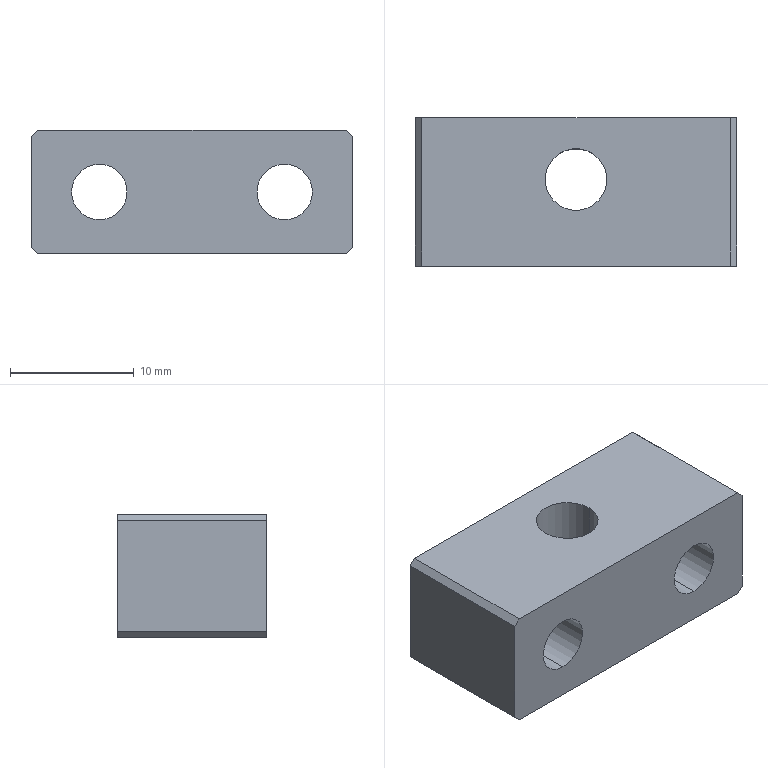Part | SolidWorks | features HoleWzd 2, Chamfer 1, Extrusion 1 | 1 solid | 22 faces | box 26 x 12 x 10 mm | volume 2220 mm3 | plane 12 | cylinder 10 | commonest cylinder face diameters 4.5 x4 8 x4 5 x2
STEP:
#1=CARTESIAN_POINT('',(-2.5,1.,-5.));
#2=VERTEX_POINT('',#1);
#3=CARTESIAN_POINT('',(2.5,1.,-5.));
#4=VERTEX_POINT('',#3);
#5=CARTESIAN_POINT('',(0.,1.,-5.));
#6=DIRECTION('',(0.,0.,1.));
#7=DIRECTION('',(1.,0.,0.));
#8=AXIS2_PLACEMENT_3D('',#5,#6,#7);
#9=CIRCLE('',#8,2.5);
#10=EDGE_CURVE('',#2,#4,#9,.T.);
#11=ORIENTED_EDGE('',*,*,#10,.F.);
#12=CARTESIAN_POINT('',(-2.5,1.,5.));
#13=VERTEX_POINT('',#12);
#14=CARTESIAN_POINT('',(-2.5,1.,5.));
#15=DIRECTION('',(0.,0.,1.));
#16=VECTOR('',#15,1000.);
#17=LINE('',#14,#16);
#18=EDGE_CURVE('',#2,#13,#17,.T.);
#19=ORIENTED_EDGE('',*,*,#18,.T.);
#20=CARTESIAN_POINT('',(2.5,1.,5.));
#21=VERTEX_POINT('',#20);
#22=CARTESIAN_POINT('',(0.,1.,5.));
#23=DIRECTION('',(0.,0.,1.));
#24=DIRECTION('',(1.,0.,0.));
#25=AXIS2_PLACEMENT_3D('',#22,#23,#24);
#26=CIRCLE('',#25,2.5);
#27=EDGE_CURVE('',#13,#21,#26,.T.);
#28=ORIENTED_EDGE('',*,*,#27,.T.);
#29=CARTESIAN_POINT('',(2.5,1.,5.));
#30=DIRECTION('',(0.,0.,1.));
#31=VECTOR('',#30,1000.);
#32=LINE('',#29,#31);
#33=EDGE_CURVE('',#4,#21,#32,.T.);
#34=ORIENTED_EDGE('',*,*,#33,.F.);
#35=EDGE_LOOP('',(#11,#19,#28,#34));
#36=FACE_OUTER_BOUND('',#35,.T.);
#37=CARTESIAN_POINT('',(0.,1.,5.));
#38=DIRECTION('',(0.,0.,1.));
#39=DIRECTION('',(1.,0.,0.));
#40=AXIS2_PLACEMENT_3D('',#37,#38,#39);
#41=CYLINDRICAL_SURFACE('',#40,2.5);
#42=ADVANCED_FACE('',(#36),#41,.F.);
#43=CARTESIAN_POINT('',(-7.5,1.4,-4.));
#44=VERTEX_POINT('',#43);
#45=CARTESIAN_POINT('',(-7.5,1.4,4.));
#46=VERTEX_POINT('',#45);
#47=CARTESIAN_POINT('',(-7.5,1.4,0.));
#48=DIRECTION('',(0.,1.,0.));
#49=DIRECTION('',(0.,0.,1.));
#50=AXIS2_PLACEMENT_3D('',#47,#48,#49);
#51=CIRCLE('',#50,4.);
#52=EDGE_CURVE('',#44,#46,#51,.T.);
#53=ORIENTED_EDGE('',*,*,#52,.F.);
#54=CARTESIAN_POINT('',(-7.5,6.,-4.));
#55=VERTEX_POINT('',#54);
#56=CARTESIAN_POINT('',(-7.5,6.,-4.));
#57=DIRECTION('',(0.,1.,0.));
#58=VECTOR('',#57,1000.);
#59=LINE('',#56,#58);
#60=EDGE_CURVE('',#44,#55,#59,.T.);
#61=ORIENTED_EDGE('',*,*,#60,.T.);
#62=CARTESIAN_POINT('',(-7.5,6.,4.));
#63=VERTEX_POINT('',#62);
#64=CARTESIAN_POINT('',(-7.5,6.,0.));
#65=DIRECTION('',(0.,1.,0.));
#66=DIRECTION('',(0.,0.,1.));
#67=AXIS2_PLACEMENT_3D('',#64,#65,#66);
#68=CIRCLE('',#67,4.);
#69=EDGE_CURVE('',#55,#63,#68,.T.);
#70=ORIENTED_EDGE('',*,*,#69,.T.);
#71=CARTESIAN_POINT('',(-7.5,6.,4.));
#72=DIRECTION('',(0.,1.,0.));
#73=VECTOR('',#72,1000.);
#74=LINE('',#71,#73);
#75=EDGE_CURVE('',#46,#63,#74,.T.);
#76=ORIENTED_EDGE('',*,*,#75,.F.);
#77=EDGE_LOOP('',(#53,#61,#70,#76));
#78=FACE_OUTER_BOUND('',#77,.T.);
#79=CARTESIAN_POINT('',(-7.5,6.,0.));
#80=DIRECTION('',(0.,1.,0.));
#81=DIRECTION('',(0.,0.,1.));
#82=AXIS2_PLACEMENT_3D('',#79,#80,#81);
#83=CYLINDRICAL_SURFACE('',#82,4.);
#84=ADVANCED_FACE('',(#78),#83,.F.);
#85=CARTESIAN_POINT('',(-7.5,-6.,-2.25));
#86=VERTEX_POINT('',#85);
#87=CARTESIAN_POINT('',(-7.5,-6.,2.25));
#88=VERTEX_POINT('',#87);
#89=CARTESIAN_POINT('',(-7.5,-6.,0.));
#90=DIRECTION('',(0.,1.,0.));
#91=DIRECTION('',(0.,0.,1.));
#92=AXIS2_PLACEMENT_3D('',#89,#90,#91);
#93=CIRCLE('',#92,2.25);
#94=EDGE_CURVE('',#86,#88,#93,.T.);
#95=ORIENTED_EDGE('',*,*,#94,.F.);
#96=CARTESIAN_POINT('',(-7.5,1.4,-2.25));
#97=VERTEX_POINT('',#96);
#98=CARTESIAN_POINT('',(-7.5,6.,-2.25));
#99=DIRECTION('',(0.,1.,0.));
#100=VECTOR('',#99,1000.);
#101=LINE('',#98,#100);
#102=EDGE_CURVE('',#86,#97,#101,.T.);
#103=ORIENTED_EDGE('',*,*,#102,.T.);
#104=CARTESIAN_POINT('',(-7.5,1.4,2.25));
#105=VERTEX_POINT('',#104);
#106=CARTESIAN_POINT('',(-7.5,1.4,0.));
#107=DIRECTION('',(0.,1.,0.));
#108=DIRECTION('',(0.,0.,1.));
#109=AXIS2_PLACEMENT_3D('',#106,#107,#108);
#110=CIRCLE('',#109,2.25);
#111=EDGE_CURVE('',#97,#105,#110,.T.);
#112=ORIENTED_EDGE('',*,*,#111,.T.);
#113=CARTESIAN_POINT('',(-7.5,6.,2.25));
#114=DIRECTION('',(0.,1.,0.));
#115=VECTOR('',#114,1000.);
#116=LINE('',#113,#115);
#117=EDGE_CURVE('',#88,#105,#116,.T.);
#118=ORIENTED_EDGE('',*,*,#117,.F.);
#119=EDGE_LOOP('',(#95,#103,#112,#118));
#120=FACE_OUTER_BOUND('',#119,.T.);
#121=CARTESIAN_POINT('',(-7.5,6.,0.));
#122=DIRECTION('',(0.,1.,0.));
#123=DIRECTION('',(0.,0.,1.));
#124=AXIS2_PLACEMENT_3D('',#121,#122,#123);
#125=CYLINDRICAL_SURFACE('',#124,2.25);
#126=ADVANCED_FACE('',(#120),#125,.F.);
#127=CARTESIAN_POINT('',(7.5,1.4,-4.));
#128=VERTEX_POINT('',#127);
#129=CARTESIAN_POINT('',(7.5,1.4,4.));
#130=VERTEX_POINT('',#129);
#131=CARTESIAN_POINT('',(7.5,1.4,0.));
#132=DIRECTION('',(0.,1.,0.));
#133=DIRECTION('',(0.,0.,1.));
#134=AXIS2_PLACEMENT_3D('',#131,#132,#133);
#135=CIRCLE('',#134,4.);
#136=EDGE_CURVE('',#128,#130,#135,.T.);
#137=ORIENTED_EDGE('',*,*,#136,.F.);
#138=CARTESIAN_POINT('',(7.5,6.,-4.));
#139=VERTEX_POINT('',#138);
#140=CARTESIAN_POINT('',(7.5,6.,-4.));
#141=DIRECTION('',(0.,1.,0.));
#142=VECTOR('',#141,1000.);
#143=LINE('',#140,#142);
#144=EDGE_CURVE('',#128,#139,#143,.T.);
#145=ORIENTED_EDGE('',*,*,#144,.T.);
#146=CARTESIAN_POINT('',(7.5,6.,4.));
#147=VERTEX_POINT('',#146);
#148=CARTESIAN_POINT('',(7.5,6.,0.));
#149=DIRECTION('',(0.,1.,0.));
#150=DIRECTION('',(0.,0.,1.));
#151=AXIS2_PLACEMENT_3D('',#148,#149,#150);
#152=CIRCLE('',#151,4.);
#153=EDGE_CURVE('',#139,#147,#152,.T.);
#154=ORIENTED_EDGE('',*,*,#153,.T.);
#155=CARTESIAN_POINT('',(7.5,6.,4.));
#156=DIRECTION('',(0.,1.,0.));
#157=VECTOR('',#156,1000.);
#158=LINE('',#155,#157);
#159=EDGE_CURVE('',#130,#147,#158,.T.);
#160=ORIENTED_EDGE('',*,*,#159,.F.);
#161=EDGE_LOOP('',(#137,#145,#154,#160));
#162=FACE_OUTER_BOUND('',#161,.T.);
#163=CARTESIAN_POINT('',(7.5,6.,0.));
#164=DIRECTION('',(0.,1.,0.));
#165=DIRECTION('',(0.,0.,1.));
#166=AXIS2_PLACEMENT_3D('',#163,#164,#165);
#167=CYLINDRICAL_SURFACE('',#166,4.);
#168=ADVANCED_FACE('',(#162),#167,.F.);
#169=CARTESIAN_POINT('',(7.5,-6.,-2.25));
#170=VERTEX_POINT('',#169);
#171=CARTESIAN_POINT('',(7.5,-6.,2.25));
#172=VERTEX_POINT('',#171);
#173=CARTESIAN_POINT('',(7.5,-6.,0.));
#174=DIRECTION('',(0.,1.,0.));
#175=DIRECTION('',(0.,0.,1.));
#176=AXIS2_PLACEMENT_3D('',#173,#174,#175);
#177=CIRCLE('',#176,2.25);
#178=EDGE_CURVE('',#170,#172,#177,.T.);
#179=ORIENTED_EDGE('',*,*,#178,.F.);
#180=CARTESIAN_POINT('',(7.5,1.4,-2.25));
#181=VERTEX_POINT('',#180);
#182=CARTESIAN_POINT('',(7.5,6.,-2.25));
#183=DIRECTION('',(0.,1.,0.));
#184=VECTOR('',#183,1000.);
#185=LINE('',#182,#184);
#186=EDGE_CURVE('',#170,#181,#185,.T.);
#187=ORIENTED_EDGE('',*,*,#186,.T.);
#188=CARTESIAN_POINT('',(7.5,1.4,2.25));
#189=VERTEX_POINT('',#188);
#190=CARTESIAN_POINT('',(7.5,1.4,0.));
#191=DIRECTION('',(0.,1.,0.));
#192=DIRECTION('',(0.,0.,1.));
#193=AXIS2_PLACEMENT_3D('',#190,#191,#192);
#194=CIRCLE('',#193,2.25);
#195=EDGE_CURVE('',#181,#189,#194,.T.);
#196=ORIENTED_EDGE('',*,*,#195,.T.);
#197=CARTESIAN_POINT('',(7.5,6.,2.25));
#198=DIRECTION('',(0.,1.,0.));
#199=VECTOR('',#198,1000.);
#200=LINE('',#197,#199);
#201=EDGE_CURVE('',#172,#189,#200,.T.);
#202=ORIENTED_EDGE('',*,*,#201,.F.);
#203=EDGE_LOOP('',(#179,#187,#196,#202));
#204=FACE_OUTER_BOUND('',#203,.T.);
#205=CARTESIAN_POINT('',(7.5,6.,0.));
#206=DIRECTION('',(0.,1.,0.));
#207=DIRECTION('',(0.,0.,1.));
#208=AXIS2_PLACEMENT_3D('',#205,#206,#207);
#209=CYLINDRICAL_SURFACE('',#208,2.25);
#210=ADVANCED_FACE('',(#204),#209,.F.);
#211=CARTESIAN_POINT('',(13.,-6.,4.5));
#212=VERTEX_POINT('',#211);
#213=CARTESIAN_POINT('',(13.,-6.,-4.5));
#214=VERTEX_POINT('',#213);
#215=CARTESIAN_POINT('',(13.,-6.,5.));
#216=DIRECTION('',(0.,0.,-1.));
#217=VECTOR('',#216,1000.);
#218=LINE('',#215,#217);
#219=EDGE_CURVE('',#212,#214,#218,.T.);
#220=ORIENTED_EDGE('',*,*,#219,.T.);
#221=CARTESIAN_POINT('',(13.,6.,-4.5));
#222=VERTEX_POINT('',#221);
#223=CARTESIAN_POINT('',(13.,6.,-4.5));
#224=DIRECTION('',(0.,1.,0.));
#225=VECTOR('',#224,1000.);
#226=LINE('',#223,#225);
#227=EDGE_CURVE('',#214,#222,#226,.T.);
#228=ORIENTED_EDGE('',*,*,#227,.T.);
#229=CARTESIAN_POINT('',(13.,6.,4.5));
#230=VERTEX_POINT('',#229);
#231=CARTESIAN_POINT('',(13.,6.,5.));
#232=DIRECTION('',(0.,0.,-1.));
#233=VECTOR('',#232,1000.);
#234=LINE('',#231,#233);
#235=EDGE_CURVE('',#230,#222,#234,.T.);
#236=ORIENTED_EDGE('',*,*,#235,.F.);
#237=CARTESIAN_POINT('',(13.,-6.,4.5));
#238=DIRECTION('',(0.,-1.,0.));
#239=VECTOR('',#238,1000.);
#240=LINE('',#237,#239);
#241=EDGE_CURVE('',#230,#212,#240,.T.);
#242=ORIENTED_EDGE('',*,*,#241,.T.);
#243=EDGE_LOOP('',(#220,#228,#236,#242));
#244=FACE_OUTER_BOUND('',#243,.T.);
#245=CARTESIAN_POINT('',(13.,6.,5.));
#246=DIRECTION('',(-1.,0.,0.));
#247=DIRECTION('',(0.,-1.,0.));
#248=AXIS2_PLACEMENT_3D('',#245,#246,#247);
#249=PLANE('',#248);
#250=ADVANCED_FACE('',(#244),#249,.F.);
#251=CARTESIAN_POINT('',(-7.5,6.,0.));
#252=DIRECTION('',(0.,1.,0.));
#253=DIRECTION('',(0.,0.,1.));
#254=AXIS2_PLACEMENT_3D('',#251,#252,#253);
#255=CIRCLE('',#254,4.);
#256=EDGE_CURVE('',#63,#55,#255,.T.);
#257=ORIENTED_EDGE('',*,*,#256,.F.);
#258=ORIENTED_EDGE('',*,*,#69,.F.);
#259=EDGE_LOOP('',(#257,#258));
#260=FACE_BOUND('',#259,.T.);
#261=CARTESIAN_POINT('',(7.5,6.,0.));
#262=DIRECTION('',(0.,1.,0.));
#263=DIRECTION('',(0.,0.,1.));
#264=AXIS2_PLACEMENT_3D('',#261,#262,#263);
#265=CIRCLE('',#264,4.);
#266=EDGE_CURVE('',#147,#139,#265,.T.);
#267=ORIENTED_EDGE('',*,*,#266,.F.);
#268=ORIENTED_EDGE('',*,*,#153,.F.);
#269=EDGE_LOOP('',(#267,#268));
#270=FACE_BOUND('',#269,.T.);
#271=CARTESIAN_POINT('',(12.5,6.,-5.));
#272=VERTEX_POINT('',#271);
#273=CARTESIAN_POINT('',(-12.5,6.,-5.));
#274=VERTEX_POINT('',#273);
#275=CARTESIAN_POINT('',(-13.,6.,-5.));
#276=DIRECTION('',(-1.,0.,0.));
#277=VECTOR('',#276,1000.);
#278=LINE('',#275,#277);
#279=EDGE_CURVE('',#272,#274,#278,.T.);
#280=ORIENTED_EDGE('',*,*,#279,.T.);
#281=CARTESIAN_POINT('',(-13.,6.,-4.5));
#282=VERTEX_POINT('',#281);
#283=CARTESIAN_POINT('',(-13.,6.,-4.5));
#284=DIRECTION('',(-0.7071,0.,0.7071));
#285=VECTOR('',#284,1000.);
#286=LINE('',#283,#285);
#287=EDGE_CURVE('',#274,#282,#286,.T.);
#288=ORIENTED_EDGE('',*,*,#287,.T.);
#289=CARTESIAN_POINT('',(-13.,6.,4.5));
#290=VERTEX_POINT('',#289);
#291=CARTESIAN_POINT('',(-13.,6.,5.));
#292=DIRECTION('',(0.,0.,-1.));
#293=VECTOR('',#292,1000.);
#294=LINE('',#291,#293);
#295=EDGE_CURVE('',#290,#282,#294,.T.);
#296=ORIENTED_EDGE('',*,*,#295,.F.);
#297=CARTESIAN_POINT('',(-12.5,6.,5.));
#298=VERTEX_POINT('',#297);
#299=CARTESIAN_POINT('',(-12.5,6.,5.));
#300=DIRECTION('',(0.7071,0.,0.7071));
#301=VECTOR('',#300,1000.);
#302=LINE('',#299,#301);
#303=EDGE_CURVE('',#290,#298,#302,.T.);
#304=ORIENTED_EDGE('',*,*,#303,.T.);
#305=CARTESIAN_POINT('',(12.5,6.,5.));
#306=VERTEX_POINT('',#305);
#307=CARTESIAN_POINT('',(-13.,6.,5.));
#308=DIRECTION('',(-1.,0.,0.));
#309=VECTOR('',#308,1000.);
#310=LINE('',#307,#309);
#311=EDGE_CURVE('',#306,#298,#310,.T.);
#312=ORIENTED_EDGE('',*,*,#311,.F.);
#313=CARTESIAN_POINT('',(12.5,6.,5.));
#314=DIRECTION('',(0.7071,0.,-0.7071));
#315=VECTOR('',#314,1000.);
#316=LINE('',#313,#315);
#317=EDGE_CURVE('',#306,#230,#316,.T.);
#318=ORIENTED_EDGE('',*,*,#317,.T.);
#319=ORIENTED_EDGE('',*,*,#235,.T.);
#320=CARTESIAN_POINT('',(13.,6.,-4.5));
#321=DIRECTION('',(-0.7071,0.,-0.7071));
#322=VECTOR('',#321,1000.);
#323=LINE('',#320,#322);
#324=EDGE_CURVE('',#222,#272,#323,.T.);
#325=ORIENTED_EDGE('',*,*,#324,.T.);
#326=EDGE_LOOP('',(#280,#288,#296,#304,#312,#318,#319,#325));
#327=FACE_OUTER_BOUND('',#326,.T.);
#328=CARTESIAN_POINT('',(-13.,6.,5.));
#329=DIRECTION('',(0.,-1.,0.));
#330=DIRECTION('',(0.,0.,-1.));
#331=AXIS2_PLACEMENT_3D('',#328,#329,#330);
#332=PLANE('',#331);
#333=ADVANCED_FACE('',(#260,#270,#327),#332,.F.);
#334=ORIENTED_EDGE('',*,*,#295,.T.);
#335=CARTESIAN_POINT('',(-13.,-6.,-4.5));
#336=VERTEX_POINT('',#335);
#337=CARTESIAN_POINT('',(-13.,6.,-4.5));
#338=DIRECTION('',(0.,-1.,0.));
#339=VECTOR('',#338,1000.);
#340=LINE('',#337,#339);
#341=EDGE_CURVE('',#282,#336,#340,.T.);
#342=ORIENTED_EDGE('',*,*,#341,.T.);
#343=CARTESIAN_POINT('',(-13.,-6.,4.5));
#344=VERTEX_POINT('',#343);
#345=CARTESIAN_POINT('',(-13.,-6.,5.));
#346=DIRECTION('',(0.,0.,-1.));
#347=VECTOR('',#346,1000.);
#348=LINE('',#345,#347);
#349=EDGE_CURVE('',#344,#336,#348,.T.);
#350=ORIENTED_EDGE('',*,*,#349,.F.);
#351=CARTESIAN_POINT('',(-13.,6.,4.5));
#352=DIRECTION('',(0.,1.,0.));
#353=VECTOR('',#352,1000.);
#354=LINE('',#351,#353);
#355=EDGE_CURVE('',#344,#290,#354,.T.);
#356=ORIENTED_EDGE('',*,*,#355,.T.);
#357=EDGE_LOOP('',(#334,#342,#350,#356));
#358=FACE_OUTER_BOUND('',#357,.T.);
#359=CARTESIAN_POINT('',(-13.,6.,5.));
#360=DIRECTION('',(1.,0.,0.));
#361=DIRECTION('',(0.,1.,0.));
#362=AXIS2_PLACEMENT_3D('',#359,#360,#361);
#363=PLANE('',#362);
#364=ADVANCED_FACE('',(#358),#363,.F.);
#365=CARTESIAN_POINT('',(-7.5,-6.,0.));
#366=DIRECTION('',(0.,1.,0.));
#367=DIRECTION('',(0.,0.,1.));
#368=AXIS2_PLACEMENT_3D('',#365,#366,#367);
#369=CIRCLE('',#368,2.25);
#370=EDGE_CURVE('',#88,#86,#369,.T.);
#371=ORIENTED_EDGE('',*,*,#370,.T.);
#372=ORIENTED_EDGE('',*,*,#94,.T.);
#373=EDGE_LOOP('',(#371,#372));
#374=FACE_BOUND('',#373,.T.);
#375=CARTESIAN_POINT('',(7.5,-6.,0.));
#376=DIRECTION('',(0.,1.,0.));
#377=DIRECTION('',(0.,0.,1.));
#378=AXIS2_PLACEMENT_3D('',#375,#376,#377);
#379=CIRCLE('',#378,2.25);
#380=EDGE_CURVE('',#172,#170,#379,.T.);
#381=ORIENTED_EDGE('',*,*,#380,.T.);
#382=ORIENTED_EDGE('',*,*,#178,.T.);
#383=EDGE_LOOP('',(#381,#382));
#384=FACE_BOUND('',#383,.T.);
#385=ORIENTED_EDGE('',*,*,#349,.T.);
#386=CARTESIAN_POINT('',(-12.5,-6.,-5.));
#387=VERTEX_POINT('',#386);
#388=CARTESIAN_POINT('',(-13.,-6.,-4.5));
#389=DIRECTION('',(0.7071,0.,-0.7071));
#390=VECTOR('',#389,1000.);
#391=LINE('',#388,#390);
#392=EDGE_CURVE('',#336,#387,#391,.T.);
#393=ORIENTED_EDGE('',*,*,#392,.T.);
#394=CARTESIAN_POINT('',(12.5,-6.,-5.));
#395=VERTEX_POINT('',#394);
#396=CARTESIAN_POINT('',(-13.,-6.,-5.));
#397=DIRECTION('',(1.,0.,0.));
#398=VECTOR('',#397,1000.);
#399=LINE('',#396,#398);
#400=EDGE_CURVE('',#387,#395,#399,.T.);
#401=ORIENTED_EDGE('',*,*,#400,.T.);
#402=CARTESIAN_POINT('',(13.,-6.,-4.5));
#403=DIRECTION('',(0.7071,0.,0.7071));
#404=VECTOR('',#403,1000.);
#405=LINE('',#402,#404);
#406=EDGE_CURVE('',#395,#214,#405,.T.);
#407=ORIENTED_EDGE('',*,*,#406,.T.);
#408=ORIENTED_EDGE('',*,*,#219,.F.);
#409=CARTESIAN_POINT('',(12.5,-6.,5.));
#410=VERTEX_POINT('',#409);
#411=CARTESIAN_POINT('',(12.5,-6.,5.));
#412=DIRECTION('',(-0.7071,0.,0.7071));
#413=VECTOR('',#412,1000.);
#414=LINE('',#411,#413);
#415=EDGE_CURVE('',#212,#410,#414,.T.);
#416=ORIENTED_EDGE('',*,*,#415,.T.);
#417=CARTESIAN_POINT('',(-12.5,-6.,5.));
#418=VERTEX_POINT('',#417);
#419=CARTESIAN_POINT('',(-13.,-6.,5.));
#420=DIRECTION('',(1.,0.,0.));
#421=VECTOR('',#420,1000.);
#422=LINE('',#419,#421);
#423=EDGE_CURVE('',#418,#410,#422,.T.);
#424=ORIENTED_EDGE('',*,*,#423,.F.);
#425=CARTESIAN_POINT('',(-12.5,-6.,5.));
#426=DIRECTION('',(-0.7071,0.,-0.7071));
#427=VECTOR('',#426,1000.);
#428=LINE('',#425,#427);
#429=EDGE_CURVE('',#418,#344,#428,.T.);
#430=ORIENTED_EDGE('',*,*,#429,.T.);
#431=EDGE_LOOP('',(#385,#393,#401,#407,#408,#416,#424,#430));
#432=FACE_OUTER_BOUND('',#431,.T.);
#433=CARTESIAN_POINT('',(-13.,-6.,5.));
#434=DIRECTION('',(0.,1.,0.));
#435=DIRECTION('',(0.,0.,1.));
#436=AXIS2_PLACEMENT_3D('',#433,#434,#435);
#437=PLANE('',#436);
#438=ADVANCED_FACE('',(#374,#384,#432),#437,.F.);
#439=CARTESIAN_POINT('',(0.,1.,5.));
#440=DIRECTION('',(0.,0.,1.));
#441=DIRECTION('',(1.,0.,0.));
#442=AXIS2_PLACEMENT_3D('',#439,#440,#441);
#443=CIRCLE('',#442,2.5);
#444=EDGE_CURVE('',#21,#13,#443,.T.);
#445=ORIENTED_EDGE('',*,*,#444,.F.);
#446=ORIENTED_EDGE('',*,*,#27,.F.);
#447=EDGE_LOOP('',(#445,#446));
#448=FACE_BOUND('',#447,.T.);
#449=ORIENTED_EDGE('',*,*,#311,.T.);
#450=CARTESIAN_POINT('',(-12.5,-6.,5.));
#451=DIRECTION('',(0.,-1.,0.));
#452=VECTOR('',#451,1000.);
#453=LINE('',#450,#452);
#454=EDGE_CURVE('',#298,#418,#453,.T.);
#455=ORIENTED_EDGE('',*,*,#454,.T.);
#456=ORIENTED_EDGE('',*,*,#423,.T.);
#457=CARTESIAN_POINT('',(12.5,6.,5.));
#458=DIRECTION('',(0.,1.,0.));
#459=VECTOR('',#458,1000.);
#460=LINE('',#457,#459);
#461=EDGE_CURVE('',#410,#306,#460,.T.);
#462=ORIENTED_EDGE('',*,*,#461,.T.);
#463=EDGE_LOOP('',(#449,#455,#456,#462));
#464=FACE_OUTER_BOUND('',#463,.T.);
#465=CARTESIAN_POINT('',(0.,0.,5.));
#466=DIRECTION('',(0.,0.,1.));
#467=DIRECTION('',(1.,0.,0.));
#468=AXIS2_PLACEMENT_3D('',#465,#466,#467);
#469=PLANE('',#468);
#470=ADVANCED_FACE('',(#448,#464),#469,.T.);
#471=CARTESIAN_POINT('',(0.,1.,-5.));
#472=DIRECTION('',(0.,0.,1.));
#473=DIRECTION('',(1.,0.,0.));
#474=AXIS2_PLACEMENT_3D('',#471,#472,#473);
#475=CIRCLE('',#474,2.5);
#476=EDGE_CURVE('',#4,#2,#475,.T.);
#477=ORIENTED_EDGE('',*,*,#476,.T.);
#478=ORIENTED_EDGE('',*,*,#10,.T.);
#479=EDGE_LOOP('',(#477,#478));
#480=FACE_BOUND('',#479,.T.);
#481=ORIENTED_EDGE('',*,*,#400,.F.);
#482=CARTESIAN_POINT('',(-12.5,0.,-5.));
#483=DIRECTION('',(0.,1.,0.));
#484=VECTOR('',#483,1000.);
#485=LINE('',#482,#484);
#486=EDGE_CURVE('',#387,#274,#485,.T.);
#487=ORIENTED_EDGE('',*,*,#486,.T.);
#488=ORIENTED_EDGE('',*,*,#279,.F.);
#489=CARTESIAN_POINT('',(12.5,0.,-5.));
#490=DIRECTION('',(0.,-1.,0.));
#491=VECTOR('',#490,1000.);
#492=LINE('',#489,#491);
#493=EDGE_CURVE('',#272,#395,#492,.T.);
#494=ORIENTED_EDGE('',*,*,#493,.T.);
#495=EDGE_LOOP('',(#481,#487,#488,#494));
#496=FACE_OUTER_BOUND('',#495,.T.);
#497=CARTESIAN_POINT('',(0.,0.,-5.));
#498=DIRECTION('',(0.,0.,1.));
#499=DIRECTION('',(1.,0.,0.));
#500=AXIS2_PLACEMENT_3D('',#497,#498,#499);
#501=PLANE('',#500);
#502=ADVANCED_FACE('',(#480,#496),#501,.F.);
#503=ORIENTED_EDGE('',*,*,#186,.F.);
#504=ORIENTED_EDGE('',*,*,#380,.F.);
#505=ORIENTED_EDGE('',*,*,#201,.T.);
#506=CARTESIAN_POINT('',(7.5,1.4,0.));
#507=DIRECTION('',(0.,1.,0.));
#508=DIRECTION('',(0.,0.,1.));
#509=AXIS2_PLACEMENT_3D('',#506,#507,#508);
#510=CIRCLE('',#509,2.25);
#511=EDGE_CURVE('',#189,#181,#510,.T.);
#512=ORIENTED_EDGE('',*,*,#511,.T.);
#513=EDGE_LOOP('',(#503,#504,#505,#512));
#514=FACE_OUTER_BOUND('',#513,.T.);
#515=CARTESIAN_POINT('',(7.5,6.,0.));
#516=DIRECTION('',(0.,1.,0.));
#517=DIRECTION('',(0.,0.,1.));
#518=AXIS2_PLACEMENT_3D('',#515,#516,#517);
#519=CYLINDRICAL_SURFACE('',#518,2.25);
#520=ADVANCED_FACE('',(#514),#519,.F.);
#521=ORIENTED_EDGE('',*,*,#511,.F.);
#522=ORIENTED_EDGE('',*,*,#195,.F.);
#523=EDGE_LOOP('',(#521,#522));
#524=FACE_BOUND('',#523,.T.);
#525=CARTESIAN_POINT('',(7.5,1.4,0.));
#526=DIRECTION('',(0.,1.,0.));
#527=DIRECTION('',(0.,0.,1.));
#528=AXIS2_PLACEMENT_3D('',#525,#526,#527);
#529=CIRCLE('',#528,4.);
#530=EDGE_CURVE('',#130,#128,#529,.T.);
#531=ORIENTED_EDGE('',*,*,#530,.T.);
#532=ORIENTED_EDGE('',*,*,#136,.T.);
#533=EDGE_LOOP('',(#531,#532));
#534=FACE_OUTER_BOUND('',#533,.T.);
#535=CARTESIAN_POINT('',(9.75,1.4,0.));
#536=DIRECTION('',(0.,-1.,0.));
#537=DIRECTION('',(0.,0.,-1.));
#538=AXIS2_PLACEMENT_3D('',#535,#536,#537);
#539=PLANE('',#538);
#540=ADVANCED_FACE('',(#524,#534),#539,.F.);
#541=ORIENTED_EDGE('',*,*,#144,.F.);
#542=ORIENTED_EDGE('',*,*,#530,.F.);
#543=ORIENTED_EDGE('',*,*,#159,.T.);
#544=ORIENTED_EDGE('',*,*,#266,.T.);
#545=EDGE_LOOP('',(#541,#542,#543,#544));
#546=FACE_OUTER_BOUND('',#545,.T.);
#547=CARTESIAN_POINT('',(7.5,6.,0.));
#548=DIRECTION('',(0.,1.,0.));
#549=DIRECTION('',(0.,0.,1.));
#550=AXIS2_PLACEMENT_3D('',#547,#548,#549);
#551=CYLINDRICAL_SURFACE('',#550,4.);
#552=ADVANCED_FACE('',(#546),#551,.F.);
#553=ORIENTED_EDGE('',*,*,#102,.F.);
#554=ORIENTED_EDGE('',*,*,#370,.F.);
#555=ORIENTED_EDGE('',*,*,#117,.T.);
#556=CARTESIAN_POINT('',(-7.5,1.4,0.));
#557=DIRECTION('',(0.,1.,0.));
#558=DIRECTION('',(0.,0.,1.));
#559=AXIS2_PLACEMENT_3D('',#556,#557,#558);
#560=CIRCLE('',#559,2.25);
#561=EDGE_CURVE('',#105,#97,#560,.T.);
#562=ORIENTED_EDGE('',*,*,#561,.T.);
#563=EDGE_LOOP('',(#553,#554,#555,#562));
#564=FACE_OUTER_BOUND('',#563,.T.);
#565=CARTESIAN_POINT('',(-7.5,6.,0.));
#566=DIRECTION('',(0.,1.,0.));
#567=DIRECTION('',(0.,0.,1.));
#568=AXIS2_PLACEMENT_3D('',#565,#566,#567);
#569=CYLINDRICAL_SURFACE('',#568,2.25);
#570=ADVANCED_FACE('',(#564),#569,.F.);
#571=ORIENTED_EDGE('',*,*,#561,.F.);
#572=ORIENTED_EDGE('',*,*,#111,.F.);
#573=EDGE_LOOP('',(#571,#572));
#574=FACE_BOUND('',#573,.T.);
#575=CARTESIAN_POINT('',(-7.5,1.4,0.));
#576=DIRECTION('',(0.,1.,0.));
#577=DIRECTION('',(0.,0.,1.));
#578=AXIS2_PLACEMENT_3D('',#575,#576,#577);
#579=CIRCLE('',#578,4.);
#580=EDGE_CURVE('',#46,#44,#579,.T.);
#581=ORIENTED_EDGE('',*,*,#580,.T.);
#582=ORIENTED_EDGE('',*,*,#52,.T.);
#583=EDGE_LOOP('',(#581,#582));
#584=FACE_OUTER_BOUND('',#583,.T.);
#585=CARTESIAN_POINT('',(-5.25,1.4,0.));
#586=DIRECTION('',(0.,-1.,0.));
#587=DIRECTION('',(0.,0.,-1.));
#588=AXIS2_PLACEMENT_3D('',#585,#586,#587);
#589=PLANE('',#588);
#590=ADVANCED_FACE('',(#574,#584),#589,.F.);
#591=ORIENTED_EDGE('',*,*,#60,.F.);
#592=ORIENTED_EDGE('',*,*,#580,.F.);
#593=ORIENTED_EDGE('',*,*,#75,.T.);
#594=ORIENTED_EDGE('',*,*,#256,.T.);
#595=EDGE_LOOP('',(#591,#592,#593,#594));
#596=FACE_OUTER_BOUND('',#595,.T.);
#597=CARTESIAN_POINT('',(-7.5,6.,0.));
#598=DIRECTION('',(0.,1.,0.));
#599=DIRECTION('',(0.,0.,1.));
#600=AXIS2_PLACEMENT_3D('',#597,#598,#599);
#601=CYLINDRICAL_SURFACE('',#600,4.);
#602=ADVANCED_FACE('',(#596),#601,.F.);
#603=ORIENTED_EDGE('',*,*,#18,.F.);
#604=ORIENTED_EDGE('',*,*,#476,.F.);
#605=ORIENTED_EDGE('',*,*,#33,.T.);
#606=ORIENTED_EDGE('',*,*,#444,.T.);
#607=EDGE_LOOP('',(#603,#604,#605,#606));
#608=FACE_OUTER_BOUND('',#607,.T.);
#609=CARTESIAN_POINT('',(0.,1.,5.));
#610=DIRECTION('',(0.,0.,1.));
#611=DIRECTION('',(1.,0.,0.));
#612=AXIS2_PLACEMENT_3D('',#609,#610,#611);
#613=CYLINDRICAL_SURFACE('',#612,2.5);
#614=ADVANCED_FACE('',(#608),#613,.F.);
#615=ORIENTED_EDGE('',*,*,#287,.F.);
#616=ORIENTED_EDGE('',*,*,#486,.F.);
#617=ORIENTED_EDGE('',*,*,#392,.F.);
#618=ORIENTED_EDGE('',*,*,#341,.F.);
#619=EDGE_LOOP('',(#615,#616,#617,#618));
#620=FACE_OUTER_BOUND('',#619,.T.);
#621=CARTESIAN_POINT('',(-13.,6.,-4.5));
#622=DIRECTION('',(0.7071,0.,0.7071));
#623=DIRECTION('',(0.,-1.,0.));
#624=AXIS2_PLACEMENT_3D('',#621,#622,#623);
#625=PLANE('',#624);
#626=ADVANCED_FACE('',(#620),#625,.F.);
#627=ORIENTED_EDGE('',*,*,#303,.F.);
#628=ORIENTED_EDGE('',*,*,#355,.F.);
#629=ORIENTED_EDGE('',*,*,#429,.F.);
#630=ORIENTED_EDGE('',*,*,#454,.F.);
#631=EDGE_LOOP('',(#627,#628,#629,#630));
#632=FACE_OUTER_BOUND('',#631,.T.);
#633=CARTESIAN_POINT('',(-12.5,0.,5.));
#634=DIRECTION('',(-0.7071,0.,0.7071));
#635=DIRECTION('',(0.,1.,0.));
#636=AXIS2_PLACEMENT_3D('',#633,#634,#635);
#637=PLANE('',#636);
#638=ADVANCED_FACE('',(#632),#637,.T.);
#639=ORIENTED_EDGE('',*,*,#406,.F.);
#640=ORIENTED_EDGE('',*,*,#493,.F.);
#641=ORIENTED_EDGE('',*,*,#324,.F.);
#642=ORIENTED_EDGE('',*,*,#227,.F.);
#643=EDGE_LOOP('',(#639,#640,#641,#642));
#644=FACE_OUTER_BOUND('',#643,.T.);
#645=CARTESIAN_POINT('',(13.,6.,-4.5));
#646=DIRECTION('',(-0.7071,0.,0.7071));
#647=DIRECTION('',(0.,1.,0.));
#648=AXIS2_PLACEMENT_3D('',#645,#646,#647);
#649=PLANE('',#648);
#650=ADVANCED_FACE('',(#644),#649,.F.);
#651=ORIENTED_EDGE('',*,*,#415,.F.);
#652=ORIENTED_EDGE('',*,*,#241,.F.);
#653=ORIENTED_EDGE('',*,*,#317,.F.);
#654=ORIENTED_EDGE('',*,*,#461,.F.);
#655=EDGE_LOOP('',(#651,#652,#653,#654));
#656=FACE_OUTER_BOUND('',#655,.T.);
#657=CARTESIAN_POINT('',(12.5,0.,5.));
#658=DIRECTION('',(0.7071,0.,0.7071));
#659=DIRECTION('',(0.,-1.,0.));
#660=AXIS2_PLACEMENT_3D('',#657,#658,#659);
#661=PLANE('',#660);
#662=ADVANCED_FACE('',(#656),#661,.T.);
#663=CLOSED_SHELL('',(#42,#84,#126,#168,#210,#250,#333,#364,#438,#470,#502,#520,#540,#552,#570,#590,#602,#614,#626,#638,#650,#662));
#664=MANIFOLD_SOLID_BREP('',#663);
#665=CARTESIAN_POINT('',(0.,0.,0.));
#666=DIRECTION('',(0.,0.,1.));
#667=DIRECTION('',(1.,0.,0.));
#668=AXIS2_PLACEMENT_3D('',#665,#666,#667);
#669=(LENGTH_UNIT()NAMED_UNIT(*)SI_UNIT(.MILLI.,.METRE.));
#670=UNCERTAINTY_MEASURE_WITH_UNIT(LENGTH_MEASURE(0.00001),#669,'','');
#671=(NAMED_UNIT(*)PLANE_ANGLE_UNIT()SI_UNIT($,.RADIAN.));
#672=(NAMED_UNIT(*)SI_UNIT($,.STERADIAN.)SOLID_ANGLE_UNIT());
#673=(GEOMETRIC_REPRESENTATION_CONTEXT(3)GLOBAL_UNCERTAINTY_ASSIGNED_CONTEXT((#670))GLOBAL_UNIT_ASSIGNED_CONTEXT((#669,#671,#672))REPRESENTATION_CONTEXT('',''));
#674=ADVANCED_BREP_SHAPE_REPRESENTATION('',(#664,#668),#673);